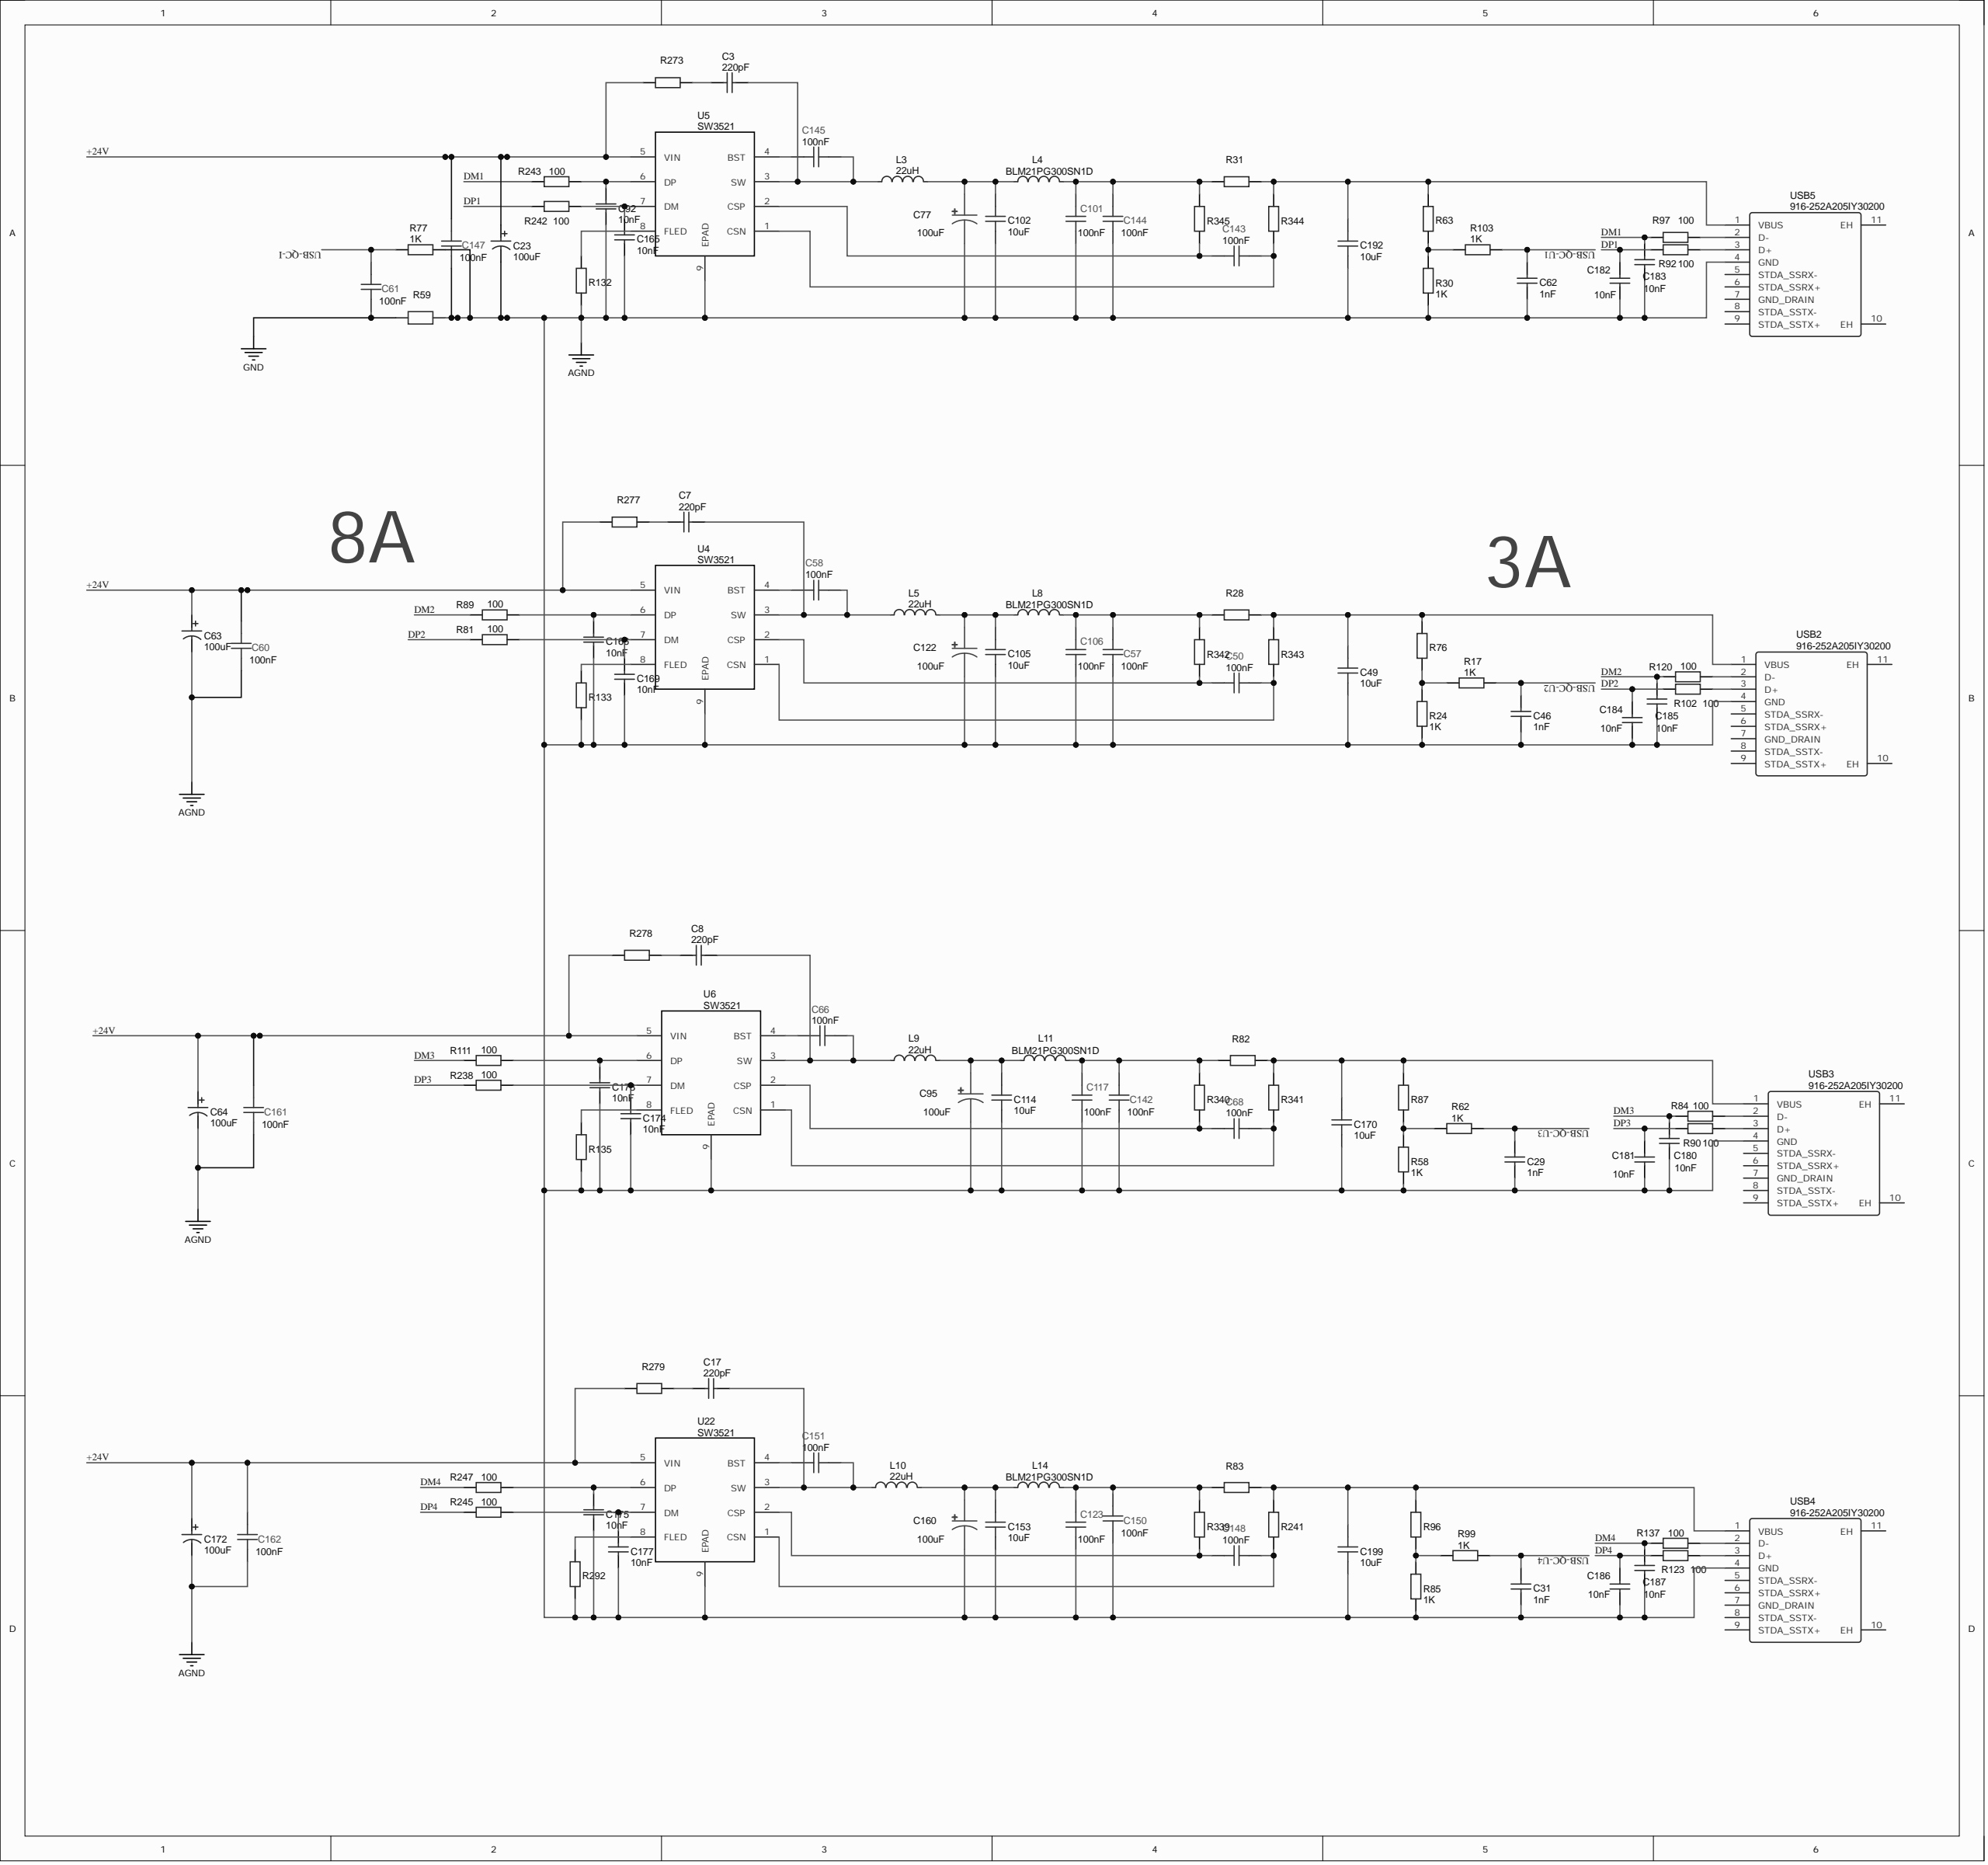Circuit board | Altium Designer | 694 parts | 423 nets | one sheet of the schematic
Parts on this sheet (reference | value | footprint):
C3 | 220pF | C0603
C7 | 220pF | C0603
C8 | 220pF | C0603
C17 | 220pF | C0603
C23 | 100uF | CAP-SMD_BD6.3-L6.6-W6.6-FD
C29 | 1nF | C0603
C31 | 1nF | C0603
C46 | 1nF | C0603
C49 | 10uF | C0603
C50 | 100nF | C0603
C57 | 100nF | C0603
C58 | 100nF | C0603
C60 | 100nF | C0603
C61 | 100nF | C0603
C62 | 1nF | C0603
C63 | 100uF | CAP-SMD_BD6.3-L6.6-W6.6-FD
C64 | 100uF | CAP-SMD_BD6.3-L6.6-W6.6-FD
C66 | 100nF | C0603
C68 | 100nF | C0603
C77 | 100uF | CAP-SMD_BD6.3-L6.6-W6.6-FD
C92 | 10nF | C0603
C95 | 100uF | CAP-SMD_BD6.3-L6.6-W6.6-FD
C101 | 100nF | C0603
C102 | 10uF | C0603
C105 | 10uF | C0603
C106 | 100nF | C0603
C114 | 10uF | C0603
C117 | 100nF | C0603
C122 | 100uF | CAP-SMD_BD6.3-L6.6-W6.6-FD
C123 | 100nF | C0603
C142 | 100nF | C0603
C143 | 100nF | C0603
C144 | 100nF | C0603
C145 | 100nF | C0603
C147 | 100nF | C0603
C148 | 100nF | C0603
C150 | 100nF | C0603
C151 | 100nF | C0603
C153 | 10uF | C0603
C160 | 100uF | CAP-SMD_BD6.3-L6.6-W6.6-FD
C161 | 100nF | C0603
C162 | 100nF | C0603
C165 | 10nF | C0603
C166 | 10nF | C0603
C169 | 10nF | C0603
C170 | 10uF | C0603
C172 | 100uF | CAP-SMD_BD6.3-L6.6-W6.6-FD
C173 | 10nF | C0603
C174 | 10nF | C0603
C175 | 10nF | C0603
C177 | 10nF | C0603
C180 | 10nF | C0603
C181 | 10nF | C0603
C182 | 10nF | C0603
C183 | 10nF | C0603
C184 | 10nF | C0603
C185 | 10nF | C0603
C186 | 10nF | C0603
C187 | 10nF | C0603
C192 | 10uF | C0603
C199 | 10uF | C0603
L3 | 22uH | IND-SMD_L7.1-W6.8
L4 | BLM21PG300SN1D | L0805
L5 | 22uH | IND-SMD_L7.1-W6.8
L8 | BLM21PG300SN1D | L0805
L9 | 22uH | IND-SMD_L7.1-W6.8
L10 | 22uH | IND-SMD_L7.1-W6.8
L11 | BLM21PG300SN1D | L0805
L14 | BLM21PG300SN1D | L0805
R17 | 1K | R0603
R24 | 1K | R0603
R28 | R2512
R30 | 1K | R0603
R31 | R2512
R58 | 1K | R0603
R59 | R2512
R62 | 1K | R0603
R63 | R0603
R76 | R0603
R77 | 1K | R0603
R81 | 100 | R0603
R82 | R2512
R83 | R2512
R84 | 100 | R0603
R85 | 1K | R0603
R87 | R0603
R89 | 100 | R0603
R90 | 100 | R0603
R92 | 100 | R0603
R96 | R0603
R97 | 100 | R0603
R99 | 1K | R0603
R102 | 100 | R0603
R103 | 1K | R0603
R111 | 100 | R0603
R120 | 100 | R0603
R123 | 100 | R0603
R132 | R0603
R133 | R0603
R135 | R0603
R137 | 100 | R0603
R238 | 100 | R0603
R241 | R0603
R242 | 100 | R0603
R243 | 100 | R0603
R245 | 100 | R0603
R247 | 100 | R0603
R273 | R0603
R277 | R0603
R278 | R0603
R279 | R0603
R292 | R0603
R339 | R0603
R340 | R0603
R341 | R0603
R342 | R0603
R343 | R0603
R344 | R0603
R345 | R0603
U4 | SW3521 | ESOP-8_L4.9-W3.9-P1.27-LS6.0-BL-EP
U5 | SW3521 | ESOP-8_L4.9-W3.9-P1.27-LS6.0-BL-EP
U6 | SW3521 | ESOP-8_L4.9-W3.9-P1.27-LS6.0-BL-EP
U22 | SW3521 | ESOP-8_L4.9-W3.9-P1.27-LS6.0-BL-EP
USB2 | 916-252A205IY30200 | USB-A-TH_916-252A205IY30200
USB3 | 916-252A205IY30200 | USB-A-TH_916-252A205IY30200
USB4 | 916-252A205IY30200 | USB-A-TH_916-252A205IY30200
USB5 | 916-252A205IY30200 | USB-A-TH_916-252A205IY30200
Nets of these parts (net: part-pin ...):
USB-QC-U4: C31-2 R99-2
USB-QC-U3: C29-2 R62-2
USB-QC-U2: C46-2 R17-2
USB-QC-U1: C62-2 R103-2
USB-QC-I: C61-2 R77-1
NetR292_2: R292-2 U22-8
NetR137_2: R137-2 USB4-2
NetR135_2: R135-2 U6-8
NetR133_2: R133-2 U4-8
NetR132_2: R132-2 U5-8
NetR123_2: R123-2 USB4-3
NetR120_2: R120-2 USB2-2
NetR102_2: R102-2 USB2-3
NetR97_2: R97-2 USB5-2
NetR92_2: R92-2 USB5-3
NetR90_2: R90-2 USB3-3
NetR85_2: R85-2 R96-2 R99-1
NetR84_2: R84-2 USB3-2
NetR58_2: R58-2 R62-1 R87-2
NetR30_2: R30-2 R63-2 R103-1
NetR17_1: R17-1 R24-2 R76-2
NetC199_2: C199-2 R83-1 R96-1 R241-1 USB4-1
NetC192_2: C192-2 R31-1 R63-1 R344-1 USB5-1
NetC177_2: C177-2 R245-2 U22-7
NetC175_2: C175-2 R247-2 U22-6
NetC174_2: C174-2 R238-2 U6-7
NetC173_2: C173-2 R111-2 U6-6
NetC170_2: C170-2 R82-1 R87-1 R341-1 USB3-1
NetC169_2: C169-2 R81-2 U4-7
NetC166_2: C166-2 R89-2 U4-6
NetC165_2: C165-2 R242-2 U5-7
NetC153_2: C153-2 C160-1 L10-2 L14-1
NetC151_2: C151-2 U22-4
NetC148_2: C148-2 R339-2 U22-2
NetC148_1: C148-1 R241-2 U22-1
NetC145_2: C145-2 U5-4
NetC143_2: C143-2 R345-2 U5-2
NetC143_1: C143-1 R344-2 U5-1
NetC123_2: C123-2 C150-2 L14-2 R83-2 R339-1
NetC117_2: C117-2 C142-2 L11-2 R82-2 R340-1
NetC105_2: C105-2 C122-1 L5-2 L8-1
NetC101_2: C101-2 C144-2 L4-2 R31-2 R345-1
NetC95_1: C95-1 C114-2 L9-2 L11-1
NetC92_2: C92-2 R243-2 U5-6
NetC77_1: C77-1 C102-2 L3-2 L4-1
NetC68_2: C68-2 R340-2 U6-2
NetC68_1: C68-1 R341-2 U6-1
NetC66_2: C66-2 U6-4
NetC58_2: C58-2 U4-4
NetC57_2: C57-2 C106-2 L8-2 R28-2 R342-1
NetC50_2: C50-2 R342-2 U4-2
NetC50_1: C50-1 R343-2 U4-1
NetC49_2: C49-2 R28-1 R76-1 R343-1 USB2-1
NetC17_2: C17-2 C151-1 L10-1 U22-3
NetC17_1: C17-1 R279-2
NetC8_2: C8-2 C66-1 L9-1 U6-3
NetC8_1: C8-1 R278-2
NetC7_2: C7-2 C58-1 L5-1 U4-3
NetC7_1: C7-1 R277-2
NetC3_2: C3-2 C145-1 L3-1 U5-3
NetC3_1: C3-1 R273-2
GND: C61-1 R59-1
DP4: C186-2 R123-1 R245-1
DP3: C181-2 R90-1 R238-1
DP2: C184-2 R81-1 R102-1
DP1: C182-2 R92-1 R242-1
DM4: C187-2 R137-1 R247-1
DM3: C180-2 R84-1 R111-1
DM2: C185-2 R89-1 R120-1
DM1: C183-2 R97-1 R243-1
AGND: C23-2 C29-1 C31-1 C46-1 C49-1 C57-1 C60-1 C62-1 C63-2 C64-2 C77-2 C92-1 C95-2 C101-1 C102-1 C105-1 C106-1 C114-1 C117-1 C122-2 C123-1 C142-1 C144-1 C147-1 C150-1 C153-1 C160-2 C161-1 C162-1 C165-1 C166-1 C169-1 C170-1 C172-2 C173-1 C174-1 C175-1 C177-1 C180-1 C181-1 C182-1 C183-1 C184-1 C185-1 C186-1 C187-1 C192-1 C199-1 R24-1 R30-1 R58-1 R59-2 R77-2 R85-1 R132-1 R133-1 R135-1 R292-1 U4-9 U5-9 U6-9 U22-9 USB2-4 USB3-4 USB4-4 USB5-4
+24V: C23-1 C60-2 C63-1 C64-1 C147-2 C161-2 C162-2 C172-1 R273-1 R277-1 R278-1 R279-1 U4-5 U5-5 U6-5 U22-5